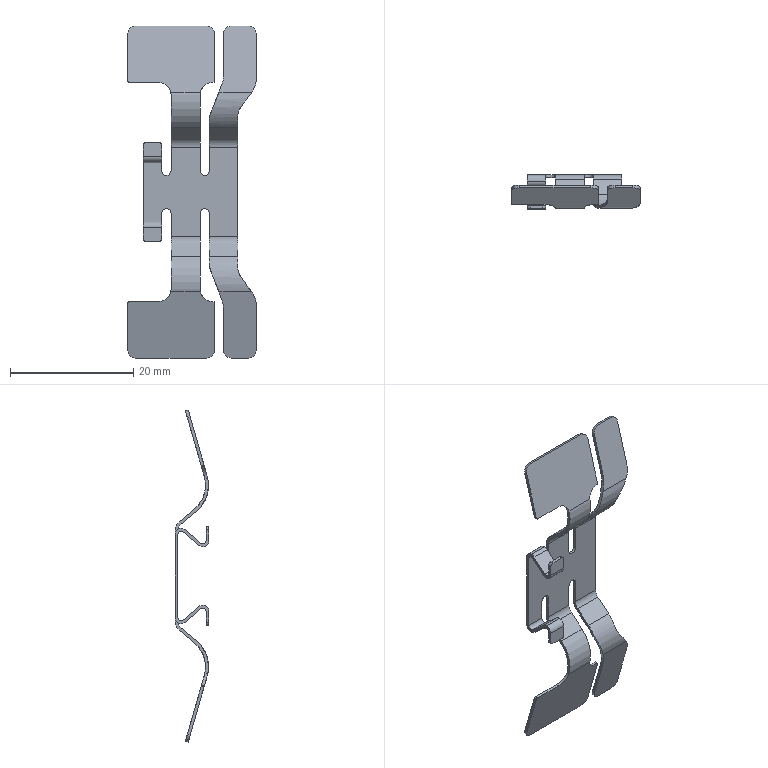Part | SolidWorks | features BaseBody 1 | 1 solid | 118 faces | box 20.8 x 5.5 x 53.8 mm | volume 398.284 mm3 | cylinder 60 | plane 58 | commonest cylinder face diameters 2.5 x8 4 x8 6 x8 1.06 x6 1.5 x6 2 x6